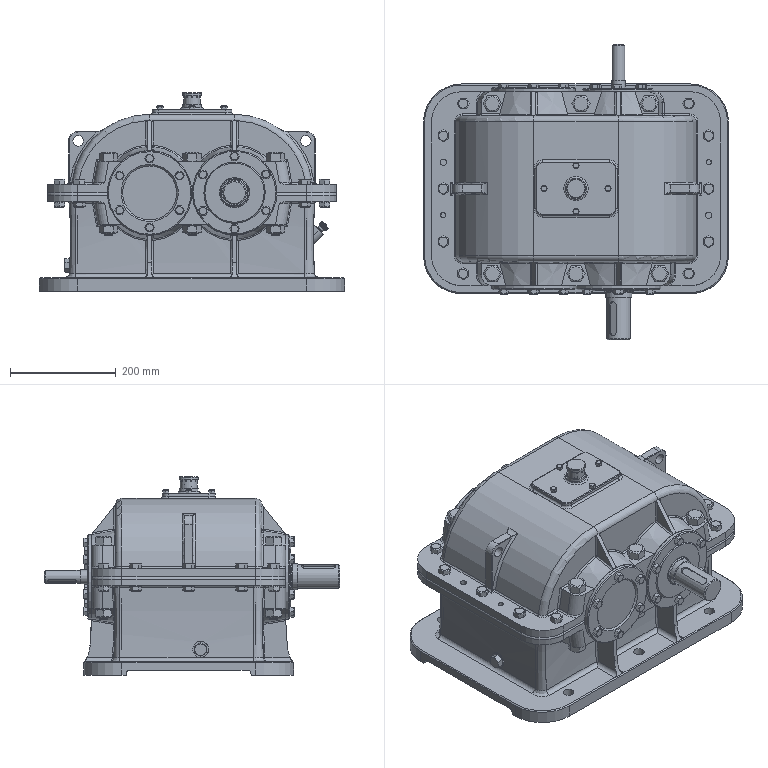Part | NX | features BREP 221, META 208, DATUM_CSYS 102, SWP104 95, EXTRACT_STRING 92, Instance Feature 88, SKETCH 68, EXTRUDE 61, CHAMFER 19, BLEND 12, CYLINDER 10, DATUM_PLANE 10, THREADS 9, CPROJ 7, BOSS 4, FSET 4, Pattern Feature 3, Mirror Feature 1, WRAP 1 | 86 solids | 7129 faces | volume 23332165 mm3 | spline 2910 | cylinder 2438 | plane 1035 | cone 643 | torus 82 | sphere 21 | commonest cylinder face diameters 8.5 x1158 18 x327 12 x171 233.325 x158 16 x107 8 x75